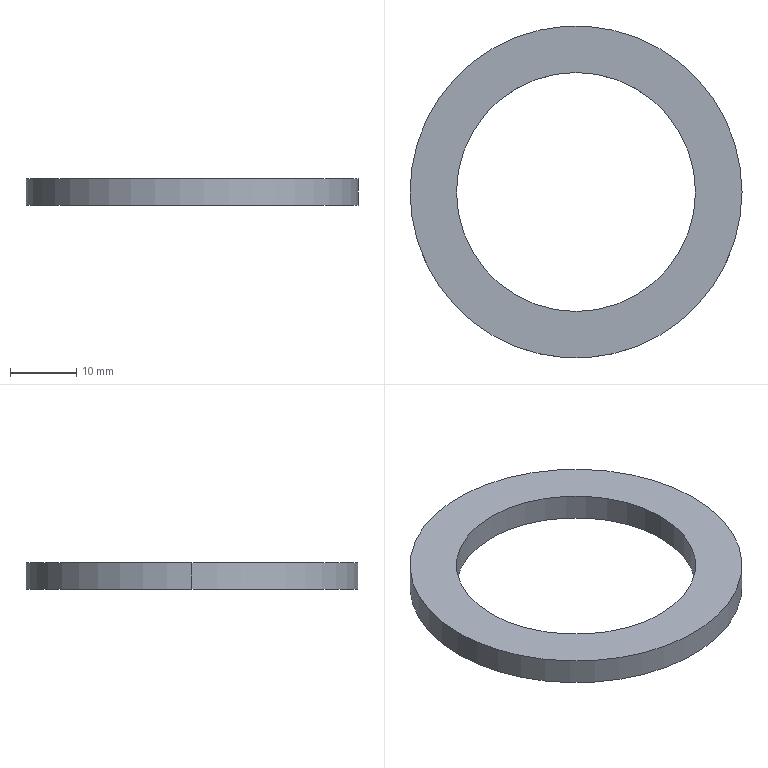Part | SolidWorks | features Extrusion 1 | 1 solid | 6 faces | box 50 x 50 x 4 mm | volume 3782 mm3 | cylinder 4 | plane 2 | commonest cylinder face diameters 36 x2 50 x2
STEP:
#1=CARTESIAN_POINT('',(-18.,0.,4.));
#2=VERTEX_POINT('',#1);
#3=CARTESIAN_POINT('',(18.,0.,4.));
#4=VERTEX_POINT('',#3);
#5=CARTESIAN_POINT('',(0.,0.,4.));
#6=DIRECTION('',(0.,0.,1.));
#7=DIRECTION('',(1.,0.,0.));
#8=AXIS2_PLACEMENT_3D('',#5,#6,#7);
#9=CIRCLE('',#8,18.);
#10=EDGE_CURVE('',#2,#4,#9,.T.);
#11=ORIENTED_EDGE('',*,*,#10,.T.);
#12=CARTESIAN_POINT('',(18.,0.,0.));
#13=VERTEX_POINT('',#12);
#14=CARTESIAN_POINT('',(18.,0.,4.));
#15=DIRECTION('',(0.,0.,-1.));
#16=VECTOR('',#15,1000.);
#17=LINE('',#14,#16);
#18=EDGE_CURVE('',#4,#13,#17,.T.);
#19=ORIENTED_EDGE('',*,*,#18,.T.);
#20=CARTESIAN_POINT('',(-18.,0.,0.));
#21=VERTEX_POINT('',#20);
#22=CARTESIAN_POINT('',(0.,0.,0.));
#23=DIRECTION('',(0.,0.,1.));
#24=DIRECTION('',(1.,0.,0.));
#25=AXIS2_PLACEMENT_3D('',#22,#23,#24);
#26=CIRCLE('',#25,18.);
#27=EDGE_CURVE('',#21,#13,#26,.T.);
#28=ORIENTED_EDGE('',*,*,#27,.F.);
#29=CARTESIAN_POINT('',(-18.,0.,4.));
#30=DIRECTION('',(0.,0.,-1.));
#31=VECTOR('',#30,1000.);
#32=LINE('',#29,#31);
#33=EDGE_CURVE('',#2,#21,#32,.T.);
#34=ORIENTED_EDGE('',*,*,#33,.F.);
#35=EDGE_LOOP('',(#11,#19,#28,#34));
#36=FACE_OUTER_BOUND('',#35,.T.);
#37=CARTESIAN_POINT('',(0.,0.,4.));
#38=DIRECTION('',(0.,0.,-1.));
#39=DIRECTION('',(-1.,0.,0.));
#40=AXIS2_PLACEMENT_3D('',#37,#38,#39);
#41=CYLINDRICAL_SURFACE('',#40,18.);
#42=ADVANCED_FACE('',(#36),#41,.F.);
#43=CARTESIAN_POINT('',(25.,0.,4.));
#44=VERTEX_POINT('',#43);
#45=CARTESIAN_POINT('',(-25.,0.,4.));
#46=VERTEX_POINT('',#45);
#47=CARTESIAN_POINT('',(0.,0.,4.));
#48=DIRECTION('',(0.,0.,1.));
#49=DIRECTION('',(1.,0.,0.));
#50=AXIS2_PLACEMENT_3D('',#47,#48,#49);
#51=CIRCLE('',#50,25.);
#52=EDGE_CURVE('',#44,#46,#51,.T.);
#53=ORIENTED_EDGE('',*,*,#52,.F.);
#54=CARTESIAN_POINT('',(25.,0.,0.));
#55=VERTEX_POINT('',#54);
#56=CARTESIAN_POINT('',(25.,0.,4.));
#57=DIRECTION('',(0.,0.,-1.));
#58=VECTOR('',#57,1000.);
#59=LINE('',#56,#58);
#60=EDGE_CURVE('',#44,#55,#59,.T.);
#61=ORIENTED_EDGE('',*,*,#60,.T.);
#62=CARTESIAN_POINT('',(-25.,0.,0.));
#63=VERTEX_POINT('',#62);
#64=CARTESIAN_POINT('',(0.,0.,0.));
#65=DIRECTION('',(0.,0.,1.));
#66=DIRECTION('',(1.,0.,0.));
#67=AXIS2_PLACEMENT_3D('',#64,#65,#66);
#68=CIRCLE('',#67,25.);
#69=EDGE_CURVE('',#55,#63,#68,.T.);
#70=ORIENTED_EDGE('',*,*,#69,.T.);
#71=CARTESIAN_POINT('',(-25.,0.,4.));
#72=DIRECTION('',(0.,0.,-1.));
#73=VECTOR('',#72,1000.);
#74=LINE('',#71,#73);
#75=EDGE_CURVE('',#46,#63,#74,.T.);
#76=ORIENTED_EDGE('',*,*,#75,.F.);
#77=EDGE_LOOP('',(#53,#61,#70,#76));
#78=FACE_OUTER_BOUND('',#77,.T.);
#79=CARTESIAN_POINT('',(0.,0.,4.));
#80=DIRECTION('',(0.,0.,-1.));
#81=DIRECTION('',(-1.,0.,0.));
#82=AXIS2_PLACEMENT_3D('',#79,#80,#81);
#83=CYLINDRICAL_SURFACE('',#82,25.);
#84=ADVANCED_FACE('',(#78),#83,.T.);
#85=CARTESIAN_POINT('',(0.,0.,4.));
#86=DIRECTION('',(0.,0.,1.));
#87=DIRECTION('',(1.,0.,0.));
#88=AXIS2_PLACEMENT_3D('',#85,#86,#87);
#89=CIRCLE('',#88,25.);
#90=EDGE_CURVE('',#46,#44,#89,.T.);
#91=ORIENTED_EDGE('',*,*,#90,.T.);
#92=ORIENTED_EDGE('',*,*,#52,.T.);
#93=EDGE_LOOP('',(#91,#92));
#94=FACE_OUTER_BOUND('',#93,.T.);
#95=ORIENTED_EDGE('',*,*,#10,.F.);
#96=CARTESIAN_POINT('',(0.,0.,4.));
#97=DIRECTION('',(0.,0.,1.));
#98=DIRECTION('',(1.,0.,0.));
#99=AXIS2_PLACEMENT_3D('',#96,#97,#98);
#100=CIRCLE('',#99,18.);
#101=EDGE_CURVE('',#4,#2,#100,.T.);
#102=ORIENTED_EDGE('',*,*,#101,.F.);
#103=EDGE_LOOP('',(#95,#102));
#104=FACE_BOUND('',#103,.T.);
#105=CARTESIAN_POINT('',(0.,0.,4.));
#106=DIRECTION('',(0.,0.,1.));
#107=DIRECTION('',(1.,0.,0.));
#108=AXIS2_PLACEMENT_3D('',#105,#106,#107);
#109=PLANE('',#108);
#110=ADVANCED_FACE('',(#94,#104),#109,.T.);
#111=CARTESIAN_POINT('',(0.,0.,0.));
#112=DIRECTION('',(0.,0.,1.));
#113=DIRECTION('',(1.,0.,0.));
#114=AXIS2_PLACEMENT_3D('',#111,#112,#113);
#115=CIRCLE('',#114,25.);
#116=EDGE_CURVE('',#63,#55,#115,.T.);
#117=ORIENTED_EDGE('',*,*,#116,.F.);
#118=ORIENTED_EDGE('',*,*,#69,.F.);
#119=EDGE_LOOP('',(#117,#118));
#120=FACE_OUTER_BOUND('',#119,.T.);
#121=ORIENTED_EDGE('',*,*,#27,.T.);
#122=CARTESIAN_POINT('',(0.,0.,0.));
#123=DIRECTION('',(0.,0.,1.));
#124=DIRECTION('',(1.,0.,0.));
#125=AXIS2_PLACEMENT_3D('',#122,#123,#124);
#126=CIRCLE('',#125,18.);
#127=EDGE_CURVE('',#13,#21,#126,.T.);
#128=ORIENTED_EDGE('',*,*,#127,.T.);
#129=EDGE_LOOP('',(#121,#128));
#130=FACE_BOUND('',#129,.T.);
#131=CARTESIAN_POINT('',(0.,0.,0.));
#132=DIRECTION('',(0.,0.,1.));
#133=DIRECTION('',(1.,0.,0.));
#134=AXIS2_PLACEMENT_3D('',#131,#132,#133);
#135=PLANE('',#134);
#136=ADVANCED_FACE('',(#120,#130),#135,.F.);
#137=ORIENTED_EDGE('',*,*,#60,.F.);
#138=ORIENTED_EDGE('',*,*,#90,.F.);
#139=ORIENTED_EDGE('',*,*,#75,.T.);
#140=ORIENTED_EDGE('',*,*,#116,.T.);
#141=EDGE_LOOP('',(#137,#138,#139,#140));
#142=FACE_OUTER_BOUND('',#141,.T.);
#143=CARTESIAN_POINT('',(0.,0.,4.));
#144=DIRECTION('',(0.,0.,-1.));
#145=DIRECTION('',(-1.,0.,0.));
#146=AXIS2_PLACEMENT_3D('',#143,#144,#145);
#147=CYLINDRICAL_SURFACE('',#146,25.);
#148=ADVANCED_FACE('',(#142),#147,.T.);
#149=ORIENTED_EDGE('',*,*,#18,.F.);
#150=ORIENTED_EDGE('',*,*,#101,.T.);
#151=ORIENTED_EDGE('',*,*,#33,.T.);
#152=ORIENTED_EDGE('',*,*,#127,.F.);
#153=EDGE_LOOP('',(#149,#150,#151,#152));
#154=FACE_OUTER_BOUND('',#153,.T.);
#155=CARTESIAN_POINT('',(0.,0.,4.));
#156=DIRECTION('',(0.,0.,-1.));
#157=DIRECTION('',(-1.,0.,0.));
#158=AXIS2_PLACEMENT_3D('',#155,#156,#157);
#159=CYLINDRICAL_SURFACE('',#158,18.);
#160=ADVANCED_FACE('',(#154),#159,.F.);
#161=CLOSED_SHELL('',(#42,#84,#110,#136,#148,#160));
#162=MANIFOLD_SOLID_BREP('',#161);
#163=CARTESIAN_POINT('',(0.,0.,0.));
#164=DIRECTION('',(0.,0.,1.));
#165=DIRECTION('',(1.,0.,0.));
#166=AXIS2_PLACEMENT_3D('',#163,#164,#165);
#167=(LENGTH_UNIT()NAMED_UNIT(*)SI_UNIT(.MILLI.,.METRE.));
#168=UNCERTAINTY_MEASURE_WITH_UNIT(LENGTH_MEASURE(0.00001),#167,'','');
#169=(NAMED_UNIT(*)PLANE_ANGLE_UNIT()SI_UNIT($,.RADIAN.));
#170=(NAMED_UNIT(*)SI_UNIT($,.STERADIAN.)SOLID_ANGLE_UNIT());
#171=(GEOMETRIC_REPRESENTATION_CONTEXT(3)GLOBAL_UNCERTAINTY_ASSIGNED_CONTEXT((#168))GLOBAL_UNIT_ASSIGNED_CONTEXT((#167,#169,#170))REPRESENTATION_CONTEXT('',''));
#172=ADVANCED_BREP_SHAPE_REPRESENTATION('',(#162,#166),#171);